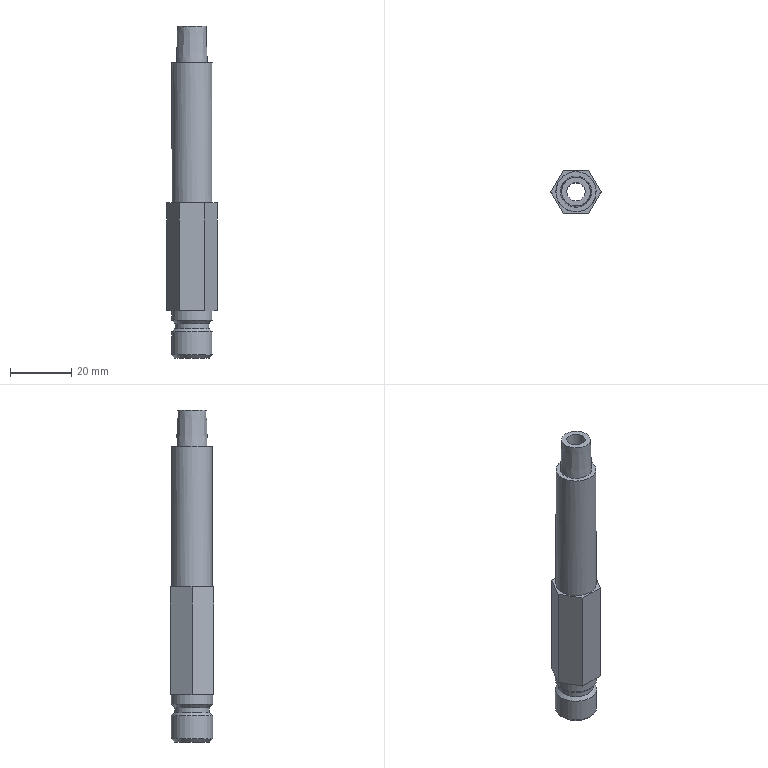Part | NX | features solid 2 | 1 solid | 20 faces | box 16.498 x 14.288 x 108.735 mm | volume 12398 mm3 | plane 11 | cylinder 5 | cone 4 | commonest cylinder face diameters 13.5 x2 6 x1 11.34 x1 13.16 x1
STEP:
#1=CARTESIAN_POINT('',(-28.58,185.,-35.));
#2=VERTEX_POINT('',#1);
#3=CARTESIAN_POINT('',(-22.,185.,-35.));
#4=DIRECTION('',(0.,0.,1.));
#5=DIRECTION('',(-1.,0.,0.));
#6=AXIS2_PLACEMENT_3D('',#3,#4,#5);
#7=CIRCLE('',#6,6.58);
#8=EDGE_CURVE('',#2,#2,#7,.F.);
#9=ORIENTED_EDGE('',*,*,#8,.F.);
#10=EDGE_LOOP('',(#9));
#11=FACE_BOUND('',#10,.T.);
#12=CARTESIAN_POINT('',(-27.079,185.,-35.));
#13=VERTEX_POINT('',#12);
#14=CARTESIAN_POINT('',(-22.,185.,-35.));
#15=DIRECTION('',(0.,0.,1.));
#16=DIRECTION('',(-1.,0.,0.));
#17=AXIS2_PLACEMENT_3D('',#14,#15,#16);
#18=CIRCLE('',#17,5.079);
#19=EDGE_CURVE('',#13,#13,#18,.F.);
#20=ORIENTED_EDGE('',*,*,#19,.T.);
#21=EDGE_LOOP('',(#20));
#22=FACE_BOUND('',#21,.T.);
#23=CARTESIAN_POINT('',(0.,152.5,-35.));
#24=DIRECTION('',(0.,0.,-1.));
#25=DIRECTION('',(-1.,0.,0.));
#26=AXIS2_PLACEMENT_3D('',#23,#24,#25);
#27=PLANE('',#26);
#28=ADVANCED_FACE('',(#11,#22),#27,.F.);
#29=CARTESIAN_POINT('',(-22.,190.67,-131.735));
#30=VERTEX_POINT('',#29);
#31=CARTESIAN_POINT('',(-22.,185.,-131.735));
#32=DIRECTION('',(0.,0.,-1.));
#33=DIRECTION('',(0.,1.,0.));
#34=AXIS2_PLACEMENT_3D('',#31,#32,#33);
#35=CIRCLE('',#34,5.67);
#36=EDGE_CURVE('',#30,#30,#35,.T.);
#37=ORIENTED_EDGE('',*,*,#36,.T.);
#38=EDGE_LOOP('',(#37));
#39=FACE_BOUND('',#38,.T.);
#40=CARTESIAN_POINT('',(-25.,185.,-131.735));
#41=VERTEX_POINT('',#40);
#42=CARTESIAN_POINT('',(-22.,185.,-131.735));
#43=DIRECTION('',(0.,0.,1.));
#44=DIRECTION('',(-1.,0.,0.));
#45=AXIS2_PLACEMENT_3D('',#42,#43,#44);
#46=CIRCLE('',#45,3.);
#47=EDGE_CURVE('',#41,#41,#46,.T.);
#48=ORIENTED_EDGE('',*,*,#47,.T.);
#49=EDGE_LOOP('',(#48));
#50=FACE_BOUND('',#49,.T.);
#51=CARTESIAN_POINT('',(-22.,185.,-131.735));
#52=DIRECTION('',(0.,0.,-1.));
#53=DIRECTION('',(0.,1.,0.));
#54=AXIS2_PLACEMENT_3D('',#51,#52,#53);
#55=PLANE('',#54);
#56=ADVANCED_FACE('',(#39,#50),#55,.T.);
#57=CARTESIAN_POINT('',(-22.,191.75,-116.235));
#58=VERTEX_POINT('',#57);
#59=CARTESIAN_POINT('',(-22.,185.,-116.235));
#60=DIRECTION('',(0.,0.,-1.));
#61=DIRECTION('',(0.,1.,0.));
#62=AXIS2_PLACEMENT_3D('',#59,#60,#61);
#63=CIRCLE('',#62,6.75);
#64=EDGE_CURVE('',#58,#58,#63,.F.);
#65=ORIENTED_EDGE('',*,*,#64,.F.);
#66=EDGE_LOOP('',(#65));
#67=FACE_BOUND('',#66,.T.);
#68=CARTESIAN_POINT('',(-22.,191.75,-119.415));
#69=VERTEX_POINT('',#68);
#70=CARTESIAN_POINT('',(-22.,185.,-119.415));
#71=DIRECTION('',(0.,0.,-1.));
#72=DIRECTION('',(0.,1.,0.));
#73=AXIS2_PLACEMENT_3D('',#70,#71,#72);
#74=CIRCLE('',#73,6.75);
#75=EDGE_CURVE('',#69,#69,#74,.T.);
#76=ORIENTED_EDGE('',*,*,#75,.F.);
#77=EDGE_LOOP('',(#76));
#78=FACE_BOUND('',#77,.T.);
#79=CARTESIAN_POINT('',(-22.,185.,-131.735));
#80=DIRECTION('',(0.,0.,-1.));
#81=DIRECTION('',(0.,1.,0.));
#82=AXIS2_PLACEMENT_3D('',#79,#80,#81);
#83=CYLINDRICAL_SURFACE('',#82,6.75);
#84=ADVANCED_FACE('',(#67,#78),#83,.T.);
#85=ORIENTED_EDGE('',*,*,#75,.T.);
#86=EDGE_LOOP('',(#85));
#87=FACE_BOUND('',#86,.T.);
#88=CARTESIAN_POINT('',(-22.,190.67,-120.495));
#89=VERTEX_POINT('',#88);
#90=CARTESIAN_POINT('',(-22.,185.,-120.495));
#91=DIRECTION('',(0.,0.,-1.));
#92=DIRECTION('',(0.,1.,0.));
#93=AXIS2_PLACEMENT_3D('',#90,#91,#92);
#94=CIRCLE('',#93,5.67);
#95=EDGE_CURVE('',#89,#89,#94,.T.);
#96=ORIENTED_EDGE('',*,*,#95,.F.);
#97=EDGE_LOOP('',(#96));
#98=FACE_BOUND('',#97,.T.);
#99=CARTESIAN_POINT('',(-22.,185.,-120.495));
#100=DIRECTION('',(0.,0.,1.));
#101=DIRECTION('',(0.,-1.,0.));
#102=AXIS2_PLACEMENT_3D('',#99,#100,#101);
#103=CONICAL_SURFACE('',#102,5.67,0.7854);
#104=ADVANCED_FACE('',(#87,#98),#103,.T.);
#105=ORIENTED_EDGE('',*,*,#95,.T.);
#106=EDGE_LOOP('',(#105));
#107=FACE_BOUND('',#106,.T.);
#108=CARTESIAN_POINT('',(-22.,190.67,-122.095));
#109=VERTEX_POINT('',#108);
#110=CARTESIAN_POINT('',(-22.,185.,-122.095));
#111=DIRECTION('',(0.,0.,-1.));
#112=DIRECTION('',(0.,1.,0.));
#113=AXIS2_PLACEMENT_3D('',#110,#111,#112);
#114=CIRCLE('',#113,5.67);
#115=EDGE_CURVE('',#109,#109,#114,.T.);
#116=ORIENTED_EDGE('',*,*,#115,.F.);
#117=EDGE_LOOP('',(#116));
#118=FACE_BOUND('',#117,.T.);
#119=CARTESIAN_POINT('',(-22.,185.,-131.735));
#120=DIRECTION('',(0.,0.,-1.));
#121=DIRECTION('',(0.,1.,0.));
#122=AXIS2_PLACEMENT_3D('',#119,#120,#121);
#123=CYLINDRICAL_SURFACE('',#122,5.67);
#124=ADVANCED_FACE('',(#107,#118),#123,.T.);
#125=ORIENTED_EDGE('',*,*,#115,.T.);
#126=EDGE_LOOP('',(#125));
#127=FACE_BOUND('',#126,.T.);
#128=CARTESIAN_POINT('',(-22.,191.75,-123.175));
#129=VERTEX_POINT('',#128);
#130=CARTESIAN_POINT('',(-22.,185.,-123.175));
#131=DIRECTION('',(0.,0.,-1.));
#132=DIRECTION('',(0.,1.,0.));
#133=AXIS2_PLACEMENT_3D('',#130,#131,#132);
#134=CIRCLE('',#133,6.75);
#135=EDGE_CURVE('',#129,#129,#134,.T.);
#136=ORIENTED_EDGE('',*,*,#135,.F.);
#137=EDGE_LOOP('',(#136));
#138=FACE_BOUND('',#137,.T.);
#139=CARTESIAN_POINT('',(-22.,185.,-123.175));
#140=DIRECTION('',(0.,0.,-1.));
#141=DIRECTION('',(0.,1.,0.));
#142=AXIS2_PLACEMENT_3D('',#139,#140,#141);
#143=CONICAL_SURFACE('',#142,6.75,0.7854);
#144=ADVANCED_FACE('',(#127,#138),#143,.T.);
#145=CARTESIAN_POINT('',(-22.,191.75,-130.655));
#146=VERTEX_POINT('',#145);
#147=CARTESIAN_POINT('',(-22.,185.,-130.655));
#148=DIRECTION('',(0.,0.,-1.));
#149=DIRECTION('',(0.,1.,0.));
#150=AXIS2_PLACEMENT_3D('',#147,#148,#149);
#151=CIRCLE('',#150,6.75);
#152=EDGE_CURVE('',#146,#146,#151,.F.);
#153=ORIENTED_EDGE('',*,*,#152,.T.);
#154=EDGE_LOOP('',(#153));
#155=FACE_BOUND('',#154,.T.);
#156=ORIENTED_EDGE('',*,*,#135,.T.);
#157=EDGE_LOOP('',(#156));
#158=FACE_BOUND('',#157,.T.);
#159=CARTESIAN_POINT('',(-22.,185.,-131.735));
#160=DIRECTION('',(0.,0.,-1.));
#161=DIRECTION('',(0.,1.,0.));
#162=AXIS2_PLACEMENT_3D('',#159,#160,#161);
#163=CYLINDRICAL_SURFACE('',#162,6.75);
#164=ADVANCED_FACE('',(#155,#158),#163,.T.);
#165=ORIENTED_EDGE('',*,*,#152,.F.);
#166=EDGE_LOOP('',(#165));
#167=FACE_BOUND('',#166,.T.);
#168=ORIENTED_EDGE('',*,*,#36,.F.);
#169=EDGE_LOOP('',(#168));
#170=FACE_BOUND('',#169,.T.);
#171=CARTESIAN_POINT('',(-22.,185.,-131.735));
#172=DIRECTION('',(0.,0.,1.));
#173=DIRECTION('',(0.,-1.,0.));
#174=AXIS2_PLACEMENT_3D('',#171,#172,#173);
#175=CONICAL_SURFACE('',#174,5.67,0.7854);
#176=ADVANCED_FACE('',(#167,#170),#175,.T.);
#177=CARTESIAN_POINT('',(-17.876,177.856,-80.929));
#178=VERTEX_POINT('',#177);
#179=CARTESIAN_POINT('',(-26.124,177.856,-80.929));
#180=VERTEX_POINT('',#179);
#181=CARTESIAN_POINT('',(-17.876,177.856,-80.929));
#182=DIRECTION('',(-1.,0.,0.));
#183=VECTOR('',#182,1000.);
#184=LINE('',#181,#183);
#185=EDGE_CURVE('',#178,#180,#184,.T.);
#186=ORIENTED_EDGE('',*,*,#185,.T.);
#187=CARTESIAN_POINT('',(-26.124,177.856,-116.235));
#188=VERTEX_POINT('',#187);
#189=CARTESIAN_POINT('',(-26.124,177.856,-116.235));
#190=DIRECTION('',(0.,0.,1.));
#191=VECTOR('',#190,1000.);
#192=LINE('',#189,#191);
#193=EDGE_CURVE('',#188,#180,#192,.T.);
#194=ORIENTED_EDGE('',*,*,#193,.F.);
#195=CARTESIAN_POINT('',(-17.876,177.856,-116.235));
#196=VERTEX_POINT('',#195);
#197=CARTESIAN_POINT('',(-17.876,177.856,-116.235));
#198=DIRECTION('',(-1.,0.,0.));
#199=VECTOR('',#198,1000.);
#200=LINE('',#197,#199);
#201=EDGE_CURVE('',#196,#188,#200,.T.);
#202=ORIENTED_EDGE('',*,*,#201,.F.);
#203=CARTESIAN_POINT('',(-17.876,177.856,-116.235));
#204=DIRECTION('',(0.,0.,1.));
#205=VECTOR('',#204,1000.);
#206=LINE('',#203,#205);
#207=EDGE_CURVE('',#196,#178,#206,.T.);
#208=ORIENTED_EDGE('',*,*,#207,.T.);
#209=EDGE_LOOP('',(#186,#194,#202,#208));
#210=FACE_BOUND('',#209,.T.);
#211=CARTESIAN_POINT('',(-17.876,177.856,-116.235));
#212=DIRECTION('',(0.,1.,0.));
#213=DIRECTION('',(1.,0.,0.));
#214=AXIS2_PLACEMENT_3D('',#211,#212,#213);
#215=PLANE('',#214);
#216=ADVANCED_FACE('',(#210),#215,.F.);
#217=CARTESIAN_POINT('',(-30.249,185.,-80.929));
#218=VERTEX_POINT('',#217);
#219=CARTESIAN_POINT('',(-26.124,177.856,-80.929));
#220=DIRECTION('',(-0.5,0.866,0.));
#221=VECTOR('',#220,1000.);
#222=LINE('',#219,#221);
#223=EDGE_CURVE('',#180,#218,#222,.T.);
#224=ORIENTED_EDGE('',*,*,#223,.T.);
#225=CARTESIAN_POINT('',(-30.249,185.,-116.235));
#226=VERTEX_POINT('',#225);
#227=CARTESIAN_POINT('',(-30.249,185.,-116.235));
#228=DIRECTION('',(0.,0.,1.));
#229=VECTOR('',#228,1000.);
#230=LINE('',#227,#229);
#231=EDGE_CURVE('',#226,#218,#230,.T.);
#232=ORIENTED_EDGE('',*,*,#231,.F.);
#233=CARTESIAN_POINT('',(-26.124,177.856,-116.235));
#234=DIRECTION('',(-0.5,0.866,0.));
#235=VECTOR('',#234,1000.);
#236=LINE('',#233,#235);
#237=EDGE_CURVE('',#188,#226,#236,.T.);
#238=ORIENTED_EDGE('',*,*,#237,.F.);
#239=ORIENTED_EDGE('',*,*,#193,.T.);
#240=EDGE_LOOP('',(#224,#232,#238,#239));
#241=FACE_BOUND('',#240,.T.);
#242=CARTESIAN_POINT('',(-26.124,177.856,-116.235));
#243=DIRECTION('',(0.866,0.5,0.));
#244=DIRECTION('',(0.5,-0.866,0.));
#245=AXIS2_PLACEMENT_3D('',#242,#243,#244);
#246=PLANE('',#245);
#247=ADVANCED_FACE('',(#241),#246,.F.);
#248=CARTESIAN_POINT('',(-26.124,192.144,-80.929));
#249=VERTEX_POINT('',#248);
#250=CARTESIAN_POINT('',(-30.249,185.,-80.929));
#251=DIRECTION('',(0.5,0.866,0.));
#252=VECTOR('',#251,1000.);
#253=LINE('',#250,#252);
#254=EDGE_CURVE('',#218,#249,#253,.T.);
#255=ORIENTED_EDGE('',*,*,#254,.T.);
#256=CARTESIAN_POINT('',(-26.124,192.144,-116.235));
#257=VERTEX_POINT('',#256);
#258=CARTESIAN_POINT('',(-26.124,192.144,-116.235));
#259=DIRECTION('',(0.,0.,1.));
#260=VECTOR('',#259,1000.);
#261=LINE('',#258,#260);
#262=EDGE_CURVE('',#257,#249,#261,.T.);
#263=ORIENTED_EDGE('',*,*,#262,.F.);
#264=CARTESIAN_POINT('',(-30.249,185.,-116.235));
#265=DIRECTION('',(0.5,0.866,0.));
#266=VECTOR('',#265,1000.);
#267=LINE('',#264,#266);
#268=EDGE_CURVE('',#226,#257,#267,.T.);
#269=ORIENTED_EDGE('',*,*,#268,.F.);
#270=ORIENTED_EDGE('',*,*,#231,.T.);
#271=EDGE_LOOP('',(#255,#263,#269,#270));
#272=FACE_BOUND('',#271,.T.);
#273=CARTESIAN_POINT('',(-30.249,185.,-116.235));
#274=DIRECTION('',(0.866,-0.5,0.));
#275=DIRECTION('',(-0.5,-0.866,0.));
#276=AXIS2_PLACEMENT_3D('',#273,#274,#275);
#277=PLANE('',#276);
#278=ADVANCED_FACE('',(#272),#277,.F.);
#279=CARTESIAN_POINT('',(-17.876,192.144,-80.929));
#280=VERTEX_POINT('',#279);
#281=CARTESIAN_POINT('',(-26.124,192.144,-80.929));
#282=DIRECTION('',(1.,0.,0.));
#283=VECTOR('',#282,1000.);
#284=LINE('',#281,#283);
#285=EDGE_CURVE('',#249,#280,#284,.T.);
#286=ORIENTED_EDGE('',*,*,#285,.T.);
#287=CARTESIAN_POINT('',(-17.876,192.144,-116.235));
#288=VERTEX_POINT('',#287);
#289=CARTESIAN_POINT('',(-17.876,192.144,-116.235));
#290=DIRECTION('',(0.,0.,1.));
#291=VECTOR('',#290,1000.);
#292=LINE('',#289,#291);
#293=EDGE_CURVE('',#288,#280,#292,.T.);
#294=ORIENTED_EDGE('',*,*,#293,.F.);
#295=CARTESIAN_POINT('',(-26.124,192.144,-116.235));
#296=DIRECTION('',(1.,0.,0.));
#297=VECTOR('',#296,1000.);
#298=LINE('',#295,#297);
#299=EDGE_CURVE('',#257,#288,#298,.T.);
#300=ORIENTED_EDGE('',*,*,#299,.F.);
#301=ORIENTED_EDGE('',*,*,#262,.T.);
#302=EDGE_LOOP('',(#286,#294,#300,#301));
#303=FACE_BOUND('',#302,.T.);
#304=CARTESIAN_POINT('',(-26.124,192.144,-116.235));
#305=DIRECTION('',(0.,-1.,0.));
#306=DIRECTION('',(-1.,0.,0.));
#307=AXIS2_PLACEMENT_3D('',#304,#305,#306);
#308=PLANE('',#307);
#309=ADVANCED_FACE('',(#303),#308,.F.);
#310=CARTESIAN_POINT('',(-13.751,185.,-80.929));
#311=VERTEX_POINT('',#310);
#312=CARTESIAN_POINT('',(-17.876,192.144,-80.929));
#313=DIRECTION('',(0.5,-0.866,0.));
#314=VECTOR('',#313,1000.);
#315=LINE('',#312,#314);
#316=EDGE_CURVE('',#280,#311,#315,.T.);
#317=ORIENTED_EDGE('',*,*,#316,.T.);
#318=CARTESIAN_POINT('',(-13.751,185.,-116.235));
#319=VERTEX_POINT('',#318);
#320=CARTESIAN_POINT('',(-13.751,185.,-116.235));
#321=DIRECTION('',(0.,0.,1.));
#322=VECTOR('',#321,1000.);
#323=LINE('',#320,#322);
#324=EDGE_CURVE('',#319,#311,#323,.T.);
#325=ORIENTED_EDGE('',*,*,#324,.F.);
#326=CARTESIAN_POINT('',(-17.876,192.144,-116.235));
#327=DIRECTION('',(0.5,-0.866,0.));
#328=VECTOR('',#327,1000.);
#329=LINE('',#326,#328);
#330=EDGE_CURVE('',#288,#319,#329,.T.);
#331=ORIENTED_EDGE('',*,*,#330,.F.);
#332=ORIENTED_EDGE('',*,*,#293,.T.);
#333=EDGE_LOOP('',(#317,#325,#331,#332));
#334=FACE_BOUND('',#333,.T.);
#335=CARTESIAN_POINT('',(-17.876,192.144,-116.235));
#336=DIRECTION('',(-0.866,-0.5,0.));
#337=DIRECTION('',(-0.5,0.866,0.));
#338=AXIS2_PLACEMENT_3D('',#335,#336,#337);
#339=PLANE('',#338);
#340=ADVANCED_FACE('',(#334),#339,.F.);
#341=CARTESIAN_POINT('',(-13.751,185.,-80.929));
#342=DIRECTION('',(-0.5,-0.866,0.));
#343=VECTOR('',#342,1000.);
#344=LINE('',#341,#343);
#345=EDGE_CURVE('',#311,#178,#344,.T.);
#346=ORIENTED_EDGE('',*,*,#345,.T.);
#347=ORIENTED_EDGE('',*,*,#207,.F.);
#348=CARTESIAN_POINT('',(-13.751,185.,-116.235));
#349=DIRECTION('',(-0.5,-0.866,0.));
#350=VECTOR('',#349,1000.);
#351=LINE('',#348,#350);
#352=EDGE_CURVE('',#319,#196,#351,.T.);
#353=ORIENTED_EDGE('',*,*,#352,.F.);
#354=ORIENTED_EDGE('',*,*,#324,.T.);
#355=EDGE_LOOP('',(#346,#347,#353,#354));
#356=FACE_BOUND('',#355,.T.);
#357=CARTESIAN_POINT('',(-13.751,185.,-116.235));
#358=DIRECTION('',(-0.866,0.5,0.));
#359=DIRECTION('',(0.5,0.866,0.));
#360=AXIS2_PLACEMENT_3D('',#357,#358,#359);
#361=PLANE('',#360);
#362=ADVANCED_FACE('',(#356),#361,.F.);
#363=ORIENTED_EDGE('',*,*,#64,.T.);
#364=EDGE_LOOP('',(#363));
#365=FACE_BOUND('',#364,.T.);
#366=ORIENTED_EDGE('',*,*,#201,.T.);
#367=ORIENTED_EDGE('',*,*,#237,.T.);
#368=ORIENTED_EDGE('',*,*,#268,.T.);
#369=ORIENTED_EDGE('',*,*,#299,.T.);
#370=ORIENTED_EDGE('',*,*,#330,.T.);
#371=ORIENTED_EDGE('',*,*,#352,.T.);
#372=EDGE_LOOP('',(#366,#367,#368,#369,#370,#371));
#373=FACE_BOUND('',#372,.T.);
#374=CARTESIAN_POINT('',(-128.8,60.,-116.235));
#375=DIRECTION('',(0.,0.,-1.));
#376=DIRECTION('',(0.,1.,0.));
#377=AXIS2_PLACEMENT_3D('',#374,#375,#376);
#378=PLANE('',#377);
#379=ADVANCED_FACE('',(#365,#373),#378,.T.);
#380=ORIENTED_EDGE('',*,*,#8,.T.);
#381=EDGE_LOOP('',(#380));
#382=FACE_BOUND('',#381,.T.);
#383=CARTESIAN_POINT('',(-22.,191.58,-80.929));
#384=VERTEX_POINT('',#383);
#385=CARTESIAN_POINT('',(-22.,185.,-80.929));
#386=DIRECTION('',(0.,0.,-1.));
#387=DIRECTION('',(0.,1.,0.));
#388=AXIS2_PLACEMENT_3D('',#385,#386,#387);
#389=CIRCLE('',#388,6.58);
#390=EDGE_CURVE('',#384,#384,#389,.T.);
#391=ORIENTED_EDGE('',*,*,#390,.F.);
#392=EDGE_LOOP('',(#391));
#393=FACE_BOUND('',#392,.T.);
#394=CARTESIAN_POINT('',(-22.,185.,-225.));
#395=DIRECTION('',(0.,0.,-1.));
#396=DIRECTION('',(0.,1.,0.));
#397=AXIS2_PLACEMENT_3D('',#394,#395,#396);
#398=CYLINDRICAL_SURFACE('',#397,6.58);
#399=ADVANCED_FACE('',(#382,#393),#398,.T.);
#400=ORIENTED_EDGE('',*,*,#390,.T.);
#401=EDGE_LOOP('',(#400));
#402=FACE_BOUND('',#401,.T.);
#403=ORIENTED_EDGE('',*,*,#185,.F.);
#404=ORIENTED_EDGE('',*,*,#345,.F.);
#405=ORIENTED_EDGE('',*,*,#316,.F.);
#406=ORIENTED_EDGE('',*,*,#285,.F.);
#407=ORIENTED_EDGE('',*,*,#254,.F.);
#408=ORIENTED_EDGE('',*,*,#223,.F.);
#409=EDGE_LOOP('',(#403,#404,#405,#406,#407,#408));
#410=FACE_BOUND('',#409,.T.);
#411=CARTESIAN_POINT('',(-28.75,185.,-80.929));
#412=DIRECTION('',(0.,0.,1.));
#413=DIRECTION('',(0.,-1.,0.));
#414=AXIS2_PLACEMENT_3D('',#411,#412,#413);
#415=PLANE('',#414);
#416=ADVANCED_FACE('',(#402,#410),#415,.T.);
#417=ORIENTED_EDGE('',*,*,#47,.F.);
#418=EDGE_LOOP('',(#417));
#419=FACE_BOUND('',#418,.T.);
#420=CARTESIAN_POINT('',(-19.,185.,-23.));
#421=VERTEX_POINT('',#420);
#422=CARTESIAN_POINT('',(-22.,185.,-23.));
#423=DIRECTION('',(0.,0.,-1.));
#424=DIRECTION('',(1.,0.,0.));
#425=AXIS2_PLACEMENT_3D('',#422,#423,#424);
#426=CIRCLE('',#425,3.);
#427=EDGE_CURVE('',#421,#421,#426,.F.);
#428=ORIENTED_EDGE('',*,*,#427,.T.);
#429=EDGE_LOOP('',(#428));
#430=FACE_BOUND('',#429,.T.);
#431=CARTESIAN_POINT('',(-22.,185.,-225.));
#432=DIRECTION('',(0.,0.,1.));
#433=DIRECTION('',(-1.,0.,0.));
#434=AXIS2_PLACEMENT_3D('',#431,#432,#433);
#435=CYLINDRICAL_SURFACE('',#434,3.);
#436=ADVANCED_FACE('',(#419,#430),#435,.F.);
#437=ORIENTED_EDGE('',*,*,#19,.F.);
#438=EDGE_LOOP('',(#437));
#439=FACE_BOUND('',#438,.T.);
#440=CARTESIAN_POINT('',(-17.296,185.,-23.));
#441=VERTEX_POINT('',#440);
#442=CARTESIAN_POINT('',(-22.,185.,-23.));
#443=DIRECTION('',(0.,0.,-1.));
#444=DIRECTION('',(1.,0.,0.));
#445=AXIS2_PLACEMENT_3D('',#442,#443,#444);
#446=CIRCLE('',#445,4.704);
#447=EDGE_CURVE('',#441,#441,#446,.F.);
#448=ORIENTED_EDGE('',*,*,#447,.F.);
#449=EDGE_LOOP('',(#448));
#450=FACE_BOUND('',#449,.T.);
#451=CARTESIAN_POINT('',(-22.,185.,-35.047));
#452=DIRECTION('',(0.,0.,-1.));
#453=DIRECTION('',(0.,1.,0.));
#454=AXIS2_PLACEMENT_3D('',#451,#452,#453);
#455=CONICAL_SURFACE('',#454,5.081,0.03124);
#456=ADVANCED_FACE('',(#439,#450),#455,.T.);
#457=ORIENTED_EDGE('',*,*,#427,.F.);
#458=EDGE_LOOP('',(#457));
#459=FACE_BOUND('',#458,.T.);
#460=ORIENTED_EDGE('',*,*,#447,.T.);
#461=EDGE_LOOP('',(#460));
#462=FACE_BOUND('',#461,.T.);
#463=CARTESIAN_POINT('',(-28.205,185.,-23.));
#464=DIRECTION('',(0.,0.,1.));
#465=DIRECTION('',(0.,-1.,0.));
#466=AXIS2_PLACEMENT_3D('',#463,#464,#465);
#467=PLANE('',#466);
#468=ADVANCED_FACE('',(#459,#462),#467,.T.);
#469=CLOSED_SHELL('',(#28,#56,#84,#104,#124,#144,#164,#176,#216,#247,#278,#309,#340,#362,#379,#399,#416,#436,#456,#468));
#470=MANIFOLD_SOLID_BREP('',#469);
#471=(LENGTH_UNIT()NAMED_UNIT(*)SI_UNIT(.MILLI.,.METRE.));
#472=UNCERTAINTY_MEASURE_WITH_UNIT(LENGTH_MEASURE(0.00001),#471,'','');
#473=(NAMED_UNIT(*)PLANE_ANGLE_UNIT()SI_UNIT($,.RADIAN.));
#474=(NAMED_UNIT(*)SI_UNIT($,.STERADIAN.)SOLID_ANGLE_UNIT());
#475=(GEOMETRIC_REPRESENTATION_CONTEXT(3)GLOBAL_UNCERTAINTY_ASSIGNED_CONTEXT((#472))GLOBAL_UNIT_ASSIGNED_CONTEXT((#471,#473,#474))REPRESENTATION_CONTEXT('',''));
#476=ADVANCED_BREP_SHAPE_REPRESENTATION('',(#470),#475);